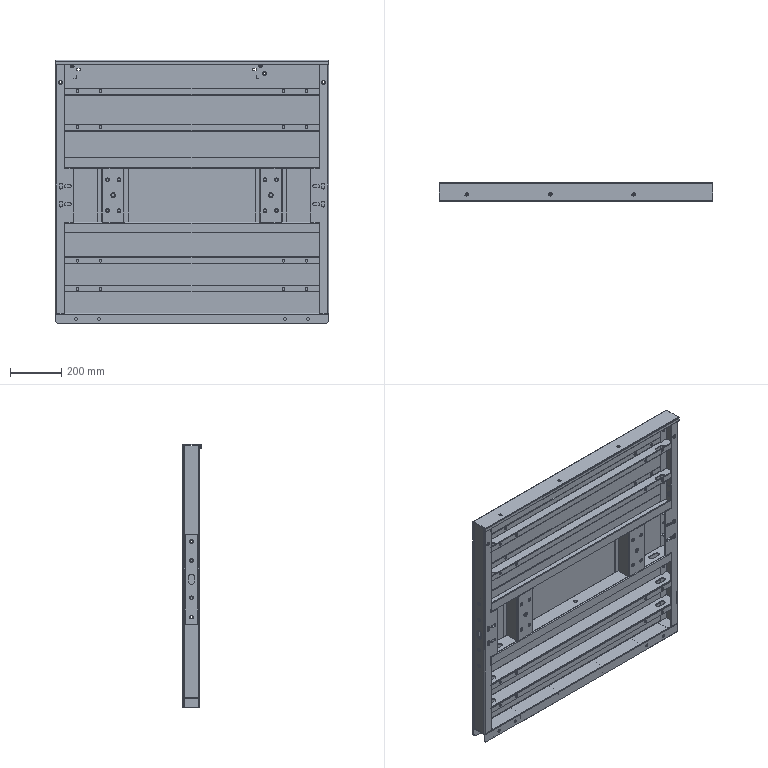Part | 48 solids | 1566 faces | box 1064 x 72 x 1025 mm | volume 7829671 mm3 | plane 900 | cylinder 522 | cone 144 | commonest cylinder face diameters 10 x86 11 x80 14.5 x48 14.75 x32 15.07 x32 0.4 x28